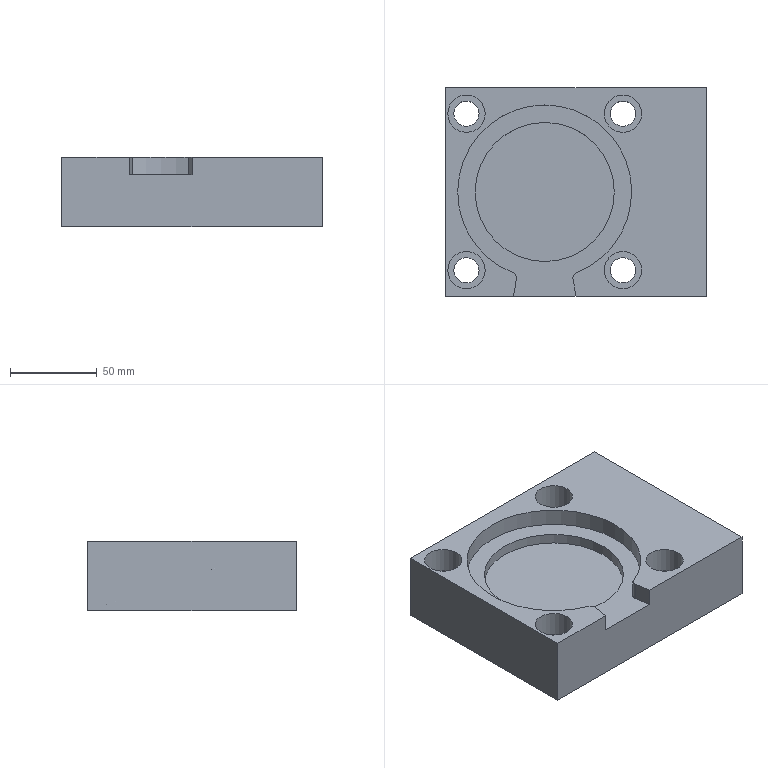NC program | NX | posted with a generic post | part box 150 x 120 x 40 mm
Lines 32 to 853 of 1997:
(HOLE_MILLING , TOOL : D10)
N56 T10 M6
N58 G54
N60 G17 G0 G90 X-63. Y45. S9500 M3
N62 G43 Z30. H10
N64 Z0.5
N66 G94 G3 X-61.563 Y43.563 R1.438 F1500.
N68 X-60.125 Y45. R1.438
N70 X-60.125 Y45. Z-0.5 I-2.875 J0.
N72 X-60.125 Y45. Z-1.5 I-2.875 J0.
N74 X-60.125 Y45. Z-2.5 I-2.875 J0.
N76 X-60.125 Y45. Z-3.5 I-2.875 J0.
N78 X-60.125 Y45. Z-4.5 I-2.875 J0.
N80 X-60.125 Y45. Z-5.5 I-2.875 J0.
N82 X-60.125 Y45. Z-6.5 I-2.875 J0.
N84 X-60.125 Y45. Z-7.5 I-2.875 J0.
N86 X-60.125 Y45. Z-8.5 I-2.875 J0.
N88 X-60.125 Y45. Z-9.5 I-2.875 J0.
N90 X-60.125 Y45. Z-10.5 I-2.875 J0.
N92 X-60.125 Y45. Z-11.5 I-2.875 J0.
N94 X-60.125 Y45. Z-12.5 I-2.875 J0.
N96 X-60.125 Y45. Z-13.5 I-2.875 J0.
N98 X-60.125 Y45. Z-14.5 I-2.875 J0.
N100 X-65.875 Y45. Z-15. I-2.875 J0.
N102 X-63. Y42.125 R2.875
N104 X-65.875 Y45. R-2.875
N106 X-64.438 Y43.563 R1.438
N108 X-63. Y45. R1.438
N110 G0 Z0.5
N112 G3 X-60.125 Y42.125 R2.875
N114 X-57.25 Y45. R2.875
N116 X-57.25 Y45. Z-0.5 I-5.75 J0.
N118 X-57.25 Y45. Z-1.5 I-5.75 J0.
N120 X-57.25 Y45. Z-2.5 I-5.75 J0.
N122 X-57.25 Y45. Z-3.5 I-5.75 J0.
N124 X-57.25 Y45. Z-4.5 I-5.75 J0.
N126 X-57.25 Y45. Z-5.5 I-5.75 J0.
N128 X-57.25 Y45. Z-6.5 I-5.75 J0.
N130 X-57.25 Y45. Z-7.5 I-5.75 J0.
N132 X-57.25 Y45. Z-8.5 I-5.75 J0.
N134 X-57.25 Y45. Z-9.5 I-5.75 J0.
N136 X-57.25 Y45. Z-10.5 I-5.75 J0.
N138 X-57.25 Y45. Z-11.5 I-5.75 J0.
N140 X-57.25 Y45. Z-12.5 I-5.75 J0.
N142 X-57.25 Y45. Z-13.5 I-5.75 J0.
N144 X-57.25 Y45. Z-14.5 I-5.75 J0.
N146 X-68.75 Y45. Z-15. I-5.75 J0.
N148 X-63. Y39.25 R5.75
N150 X-68.75 Y45. R-5.75
N152 X-65.875 Y42.125 R2.875
N154 X-63. Y45. R2.875
N156 G0 Z30.
N158 X27.
N160 Z0.5
N162 G3 X28.438 Y43.563 R1.438
N164 X29.875 Y45. R1.438
N166 X29.875 Y45. Z-0.5 I-2.875 J0.
N168 X29.875 Y45. Z-1.5 I-2.875 J0.
N170 X29.875 Y45. Z-2.5 I-2.875 J0.
N172 X29.875 Y45. Z-3.5 I-2.875 J0.
N174 X29.875 Y45. Z-4.5 I-2.875 J0.
N176 X29.875 Y45. Z-5.5 I-2.875 J0.
N178 X29.875 Y45. Z-6.5 I-2.875 J0.
N180 X29.875 Y45. Z-7.5 I-2.875 J0.
N182 X29.875 Y45. Z-8.5 I-2.875 J0.
N184 X29.875 Y45. Z-9.5 I-2.875 J0.
N186 X29.875 Y45. Z-10.5 I-2.875 J0.
N188 X29.875 Y45. Z-11.5 I-2.875 J0.
N190 X29.875 Y45. Z-12.5 I-2.875 J0.
N192 X29.875 Y45. Z-13.5 I-2.875 J0.
N194 X29.875 Y45. Z-14.5 I-2.875 J0.
N196 X24.125 Y45. Z-15. I-2.875 J0.
N198 X27. Y42.125 R2.875
N200 X24.125 Y45. R-2.875
N202 X25.563 Y43.563 R1.438
N204 X27. Y45. R1.438
N206 G0 Z0.5
N208 G3 X29.875 Y42.125 R2.875
N210 X32.75 Y45. R2.875
N212 X32.75 Y45. Z-0.5 I-5.75 J0.
N214 X32.75 Y45. Z-1.5 I-5.75 J0.
N216 X32.75 Y45. Z-2.5 I-5.75 J0.
N218 X32.75 Y45. Z-3.5 I-5.75 J0.
N220 X32.75 Y45. Z-4.5 I-5.75 J0.
N222 X32.75 Y45. Z-5.5 I-5.75 J0.
N224 X32.75 Y45. Z-6.5 I-5.75 J0.
N226 X32.75 Y45. Z-7.5 I-5.75 J0.
N228 X32.75 Y45. Z-8.5 I-5.75 J0.
N230 X32.75 Y45. Z-9.5 I-5.75 J0.
N232 X32.75 Y45. Z-10.5 I-5.75 J0.
N234 X32.75 Y45. Z-11.5 I-5.75 J0.
N236 X32.75 Y45. Z-12.5 I-5.75 J0.
N238 X32.75 Y45. Z-13.5 I-5.75 J0.
N240 X32.75 Y45. Z-14.5 I-5.75 J0.
N242 X21.25 Y45. Z-15. I-5.75 J0.
N244 X27. Y39.25 R5.75
N246 X21.25 Y45. R-5.75
N248 X24.125 Y42.125 R2.875
N250 X27. Y45. R2.875
N252 G0 Z30.
N254 Y-45.
N256 Z0.5
N258 G3 X28.438 Y-46.438 R1.438
N260 X29.875 Y-45. R1.438
N262 X29.875 Y-45. Z-0.5 I-2.875 J0.
N264 X29.875 Y-45. Z-1.5 I-2.875 J0.
N266 X29.875 Y-45. Z-2.5 I-2.875 J0.
N268 X29.875 Y-45. Z-3.5 I-2.875 J0.
N270 X29.875 Y-45. Z-4.5 I-2.875 J0.
N272 X29.875 Y-45. Z-5.5 I-2.875 J0.
N274 X29.875 Y-45. Z-6.5 I-2.875 J0.
N276 X29.875 Y-45. Z-7.5 I-2.875 J0.
N278 X29.875 Y-45. Z-8.5 I-2.875 J0.
N280 X29.875 Y-45. Z-9.5 I-2.875 J0.
N282 X29.875 Y-45. Z-10.5 I-2.875 J0.
N284 X29.875 Y-45. Z-11.5 I-2.875 J0.
N286 X29.875 Y-45. Z-12.5 I-2.875 J0.
N288 X29.875 Y-45. Z-13.5 I-2.875 J0.
N290 X29.875 Y-45. Z-14.5 I-2.875 J0.
N292 X24.125 Y-45. Z-15. I-2.875 J0.
N294 X27. Y-47.875 R2.875
N296 X24.125 Y-45. R-2.875
N298 X25.563 Y-46.438 R1.438
N300 X27. Y-45. R1.438
N302 G0 Z0.5
N304 G3 X29.875 Y-47.875 R2.875
N306 X32.75 Y-45. R2.875
N308 X32.75 Y-45. Z-0.5 I-5.75 J0.
N310 X32.75 Y-45. Z-1.5 I-5.75 J0.
N312 X32.75 Y-45. Z-2.5 I-5.75 J0.
N314 X32.75 Y-45. Z-3.5 I-5.75 J0.
N316 X32.75 Y-45. Z-4.5 I-5.75 J0.
N318 X32.75 Y-45. Z-5.5 I-5.75 J0.
N320 X32.75 Y-45. Z-6.5 I-5.75 J0.
N322 X32.75 Y-45. Z-7.5 I-5.75 J0.
N324 X32.75 Y-45. Z-8.5 I-5.75 J0.
N326 X32.75 Y-45. Z-9.5 I-5.75 J0.
N328 X32.75 Y-45. Z-10.5 I-5.75 J0.
N330 X32.75 Y-45. Z-11.5 I-5.75 J0.
N332 X32.75 Y-45. Z-12.5 I-5.75 J0.
N334 X32.75 Y-45. Z-13.5 I-5.75 J0.
N336 X32.75 Y-45. Z-14.5 I-5.75 J0.
N338 X21.25 Y-45. Z-15. I-5.75 J0.
N340 X27. Y-50.75 R5.75
N342 X21.25 Y-45. R-5.75
N344 X24.125 Y-47.875 R2.875
N346 X27. Y-45. R2.875
N348 G0 Z30.
N350 X-63.
N352 Z0.5
N354 G3 X-61.563 Y-46.438 R1.438
N356 X-60.125 Y-45. R1.438
N358 X-60.125 Y-45. Z-0.5 I-2.875 J0.
N360 X-60.125 Y-45. Z-1.5 I-2.875 J0.
N362 X-60.125 Y-45. Z-2.5 I-2.875 J0.
N364 X-60.125 Y-45. Z-3.5 I-2.875 J0.
N366 X-60.125 Y-45. Z-4.5 I-2.875 J0.
N368 X-60.125 Y-45. Z-5.5 I-2.875 J0.
N370 X-60.125 Y-45. Z-6.5 I-2.875 J0.
N372 X-60.125 Y-45. Z-7.5 I-2.875 J0.
N374 X-60.125 Y-45. Z-8.5 I-2.875 J0.
N376 X-60.125 Y-45. Z-9.5 I-2.875 J0.
N378 X-60.125 Y-45. Z-10.5 I-2.875 J0.
N380 X-60.125 Y-45. Z-11.5 I-2.875 J0.
N382 X-60.125 Y-45. Z-12.5 I-2.875 J0.
N384 X-60.125 Y-45. Z-13.5 I-2.875 J0.
N386 X-60.125 Y-45. Z-14.5 I-2.875 J0.
N388 X-65.875 Y-45. Z-15. I-2.875 J0.
N390 X-63. Y-47.875 R2.875
N392 X-65.875 Y-45. R-2.875
N394 X-64.438 Y-46.438 R1.438
N396 X-63. Y-45. R1.438
N398 G0 Z0.5
N400 G3 X-60.125 Y-47.875 R2.875
N402 X-57.25 Y-45. R2.875
N404 X-57.25 Y-45. Z-0.5 I-5.75 J0.
N406 X-57.25 Y-45. Z-1.5 I-5.75 J0.
N408 X-57.25 Y-45. Z-2.5 I-5.75 J0.
N410 X-57.25 Y-45. Z-3.5 I-5.75 J0.
N412 X-57.25 Y-45. Z-4.5 I-5.75 J0.
N414 X-57.25 Y-45. Z-5.5 I-5.75 J0.
N416 X-57.25 Y-45. Z-6.5 I-5.75 J0.
N418 X-57.25 Y-45. Z-7.5 I-5.75 J0.
N420 X-57.25 Y-45. Z-8.5 I-5.75 J0.
N422 X-57.25 Y-45. Z-9.5 I-5.75 J0.
N424 X-57.25 Y-45. Z-10.5 I-5.75 J0.
N426 X-57.25 Y-45. Z-11.5 I-5.75 J0.
N428 X-57.25 Y-45. Z-12.5 I-5.75 J0.
N430 X-57.25 Y-45. Z-13.5 I-5.75 J0.
N432 X-57.25 Y-45. Z-14.5 I-5.75 J0.
N434 X-68.75 Y-45. Z-15. I-5.75 J0.
N436 X-63. Y-50.75 R5.75
N438 X-68.75 Y-45. R-5.75
N440 X-65.875 Y-47.875 R2.875
N442 X-63. Y-45. R2.875
N444 G0 Z30.
(FLOOR_WALL , TOOL : D10)
N446 X-16.17 Y2.26
N448 Z1.5
N450 G1 X-16.818 Y2.681 Z1.459 F1000.
N452 X-17.725 Y2.917 Z1.41
N454 X-18.66 Y2.855 Z1.361
N456 X-19.049 Y2.703 Z1.339
N458 X-19.439 Y2.552 Z1.317
N460 X-20.171 Y1.967 Z1.268
N462 X-20.681 Y1.182 Z1.219
N464 X-20.917 Y0.275 Z1.17
N466 X-20.855 Y-0.66 Z1.121
N468 X-20.703 Y-1.049 Z1.099
N470 X-20.552 Y-1.439 Z1.077
N472 X-20.072 Y-2.072 Z1.036
N474 X-19.439 Y-2.552 Z0.994
N476 X-18. Y-3.125 Z0.913
N478 X-16.561 Y-2.552 Z0.832
N480 X-15.829 Y-1.967 Z0.783
N482 X-15.319 Y-1.182 Z0.733
N484 X-15.083 Y-0.275 Z0.684
N486 X-15.145 Y0.66 Z0.635
N488 X-15.297 Y1.049 Z0.613
N490 X-15.448 Y1.439 Z0.591
N492 X-16.033 Y2.171 Z0.542
N494 X-16.818 Y2.681 Z0.493
N496 X-17.725 Y2.917 Z0.444
N498 X-18.66 Y2.855 Z0.395
N500 X-19.049 Y2.703 Z0.373
N502 X-19.439 Y2.552 Z0.351
N504 X-20.171 Y1.967 Z0.302
N506 X-20.681 Y1.182 Z0.253
N508 X-20.917 Y0.275 Z0.204
N510 X-20.855 Y-0.66 Z0.155
N512 X-20.703 Y-1.049 Z0.133
N514 X-20.552 Y-1.439 Z0.111
N516 X-20.072 Y-2.072 Z0.069
N518 X-19.439 Y-2.552 Z0.028
N520 X-18. Y-3.125 Z-0.053
N522 X-16.561 Y-2.552 Z-0.135
N524 X-15.829 Y-1.967 Z-0.184
N526 X-15.319 Y-1.182 Z-0.233
N528 X-15.083 Y-0.275 Z-0.282
N530 X-15.145 Y0.66 Z-0.331
N532 X-15.297 Y1.049 Z-0.353
N534 X-15.448 Y1.439 Z-0.375
N536 X-16.033 Y2.171 Z-0.424
N538 X-16.818 Y2.681 Z-0.473
N540 X-17.725 Y2.917 Z-0.522
N542 X-18.66 Y2.855 Z-0.571
N544 X-19.049 Y2.703 Z-0.593
N546 X-19.439 Y2.552 Z-0.615
N548 X-20.171 Y1.967 Z-0.664
N550 X-20.681 Y1.182 Z-0.713
N552 X-20.917 Y0.275 Z-0.762
N554 X-20.855 Y-0.66 Z-0.811
N556 X-20.703 Y-1.049 Z-0.833
N558 X-20.552 Y-1.439 Z-0.855
N560 X-20.072 Y-2.072 Z-0.897
N562 X-19.439 Y-2.552 Z-0.938
N564 X-18.524 Y-2.911 Z-0.99
N566 G2 X-18. Y-3.125 R50.1 F3500.
N568 X-16.951 Y-2.703 R50.1
N570 G3 X-19.049 Y-2.703 R-2.9
N572 G2 X-18.524 Y-2.911 R50.1
N574 G1 X-20.758 Y-8.48
N576 G2 X-18. Y-9.697 R44.1
N578 X-14.779 Y-8.297 R44.1
N580 G3 X-21.221 Y-8.297 R-8.9
N582 G2 X-20.758 Y-8.48 R44.1
N584 G1 X-22.992 Y-14.048
N586 G2 X-18. Y-16.487 R38.1
N588 X-12.608 Y-13.89 R38.1
N590 G3 X-23.392 Y-13.89 R-14.9
N592 G2 X-22.992 Y-14.048 R38.1
N594 G1 X-25.226 Y-19.617
N596 G2 X-18. Y-23.667 R32.1
N598 X-10.437 Y-19.484 R32.1
N600 G3 X-25.563 Y-19.484 R-20.9
N602 G2 X-25.226 Y-19.617 R32.1
N604 G1 X-27.46 Y-25.185
N606 G2 X-18. Y-31.706 R26.1
N608 X-8.266 Y-25.077 R26.1
N610 G3 X-27.734 Y-25.077 R-26.9
N612 G2 X-27.46 Y-25.185 R26.1
N614 G1 X-29.694 Y-30.754
N616 G2 X-18. Y-43.393 R20.1
N618 G1 Y-52.243
N620 Y-43.393
N622 G2 X-6.095 Y-30.67 R20.1
N624 G3 X-29.905 Y-30.67 R-32.9
N626 G2 X-29.694 Y-30.754 R20.1
N628 G1 X-31.928 Y-36.322
N630 G2 X-23.293 Y-51.857 R14.1
N632 G1 X-24.552 Y-59.
N634 X-11.448
N636 X-12.707 Y-51.856
N638 G2 X-3.924 Y-36.264 R14.1
N640 G3 X-32.076 Y-36.264 R-38.9
N642 G1 X-31.928 Y-36.322
N644 X-34.163 Y-41.891
N646 G2 X-29.202 Y-50.815 R8.1
N648 G1 X-31.703 Y-65.
N650 X-4.297
N652 X-6.798 Y-50.815
N654 G2 X-1.752 Y-41.857 R8.1
N656 G3 X-34.248 Y-41.857 R-44.9
N658 G1 X-34.163 Y-41.891
N660 Z0.51
N662 G0 Z3.
N664 X-16.17 Y2.26
N666 Z0.51
N668 G1 X-16.818 Y2.681 Z0.469 F1000.
N670 X-17.725 Y2.917 Z0.42
N672 X-18.66 Y2.855 Z0.371
N674 X-19.049 Y2.703 Z0.349
N676 X-19.439 Y2.552 Z0.327
N678 X-20.171 Y1.967 Z0.278
N680 X-20.681 Y1.182 Z0.229
N682 X-20.917 Y0.275 Z0.18
N684 X-20.855 Y-0.66 Z0.131
N686 X-20.703 Y-1.049 Z0.109
N688 X-20.552 Y-1.439 Z0.087
N690 X-20.072 Y-2.072 Z0.046
N692 X-19.439 Y-2.552 Z0.004
N694 X-18. Y-3.125 Z-0.077
N696 X-16.561 Y-2.552 Z-0.158
N698 X-15.829 Y-1.967 Z-0.207
N700 X-15.319 Y-1.182 Z-0.257
N702 X-15.083 Y-0.275 Z-0.306
N704 X-15.145 Y0.66 Z-0.355
N706 X-15.297 Y1.049 Z-0.377
N708 X-15.448 Y1.439 Z-0.399
N710 X-16.033 Y2.171 Z-0.448
N712 X-16.818 Y2.681 Z-0.497
N714 X-17.725 Y2.917 Z-0.546
N716 X-18.66 Y2.855 Z-0.595
N718 X-19.049 Y2.703 Z-0.617
N720 X-19.439 Y2.552 Z-0.639
N722 X-20.171 Y1.967 Z-0.688
N724 X-20.681 Y1.182 Z-0.737
N726 X-20.917 Y0.275 Z-0.786
N728 X-20.855 Y-0.66 Z-0.835
N730 X-20.703 Y-1.049 Z-0.857
N732 X-20.552 Y-1.439 Z-0.879
N734 X-20.072 Y-2.072 Z-0.921
N736 X-19.439 Y-2.552 Z-0.962
N738 X-18. Y-3.125 Z-1.043
N740 X-16.561 Y-2.552 Z-1.125
N742 X-15.829 Y-1.967 Z-1.174
N744 X-15.319 Y-1.182 Z-1.223
N746 X-15.083 Y-0.275 Z-1.272
N748 X-15.145 Y0.66 Z-1.321
N750 X-15.297 Y1.049 Z-1.343
N752 X-15.448 Y1.439 Z-1.365
N754 X-16.033 Y2.171 Z-1.414
N756 X-16.818 Y2.681 Z-1.463
N758 X-17.725 Y2.917 Z-1.512
N760 X-18.66 Y2.855 Z-1.561
N762 X-19.049 Y2.703 Z-1.583
N764 X-19.439 Y2.552 Z-1.605
N766 X-20.171 Y1.967 Z-1.654
N768 X-20.681 Y1.182 Z-1.703
N770 X-20.917 Y0.275 Z-1.752
N772 X-20.855 Y-0.66 Z-1.801
N774 X-20.703 Y-1.049 Z-1.823
N776 X-20.552 Y-1.439 Z-1.845
N778 X-20.072 Y-2.072 Z-1.887
N780 X-19.439 Y-2.552 Z-1.928
N782 X-18.524 Y-2.911 Z-1.98
N784 G2 X-18. Y-3.125 R50.1 F3500.
N786 X-16.951 Y-2.703 R50.1
N788 G3 X-19.049 Y-2.703 R-2.9
N790 G2 X-18.524 Y-2.911 R50.1
N792 G1 X-20.758 Y-8.48
N794 G2 X-18. Y-9.697 R44.1
N796 X-14.779 Y-8.297 R44.1
N798 G3 X-21.221 Y-8.297 R-8.9
N800 G2 X-20.758 Y-8.48 R44.1
N802 G1 X-22.992 Y-14.048
N804 G2 X-18. Y-16.487 R38.1
N806 X-12.608 Y-13.89 R38.1
N808 G3 X-23.392 Y-13.89 R-14.9
N810 G2 X-22.992 Y-14.048 R38.1
N812 G1 X-25.226 Y-19.617
N814 G2 X-18. Y-23.667 R32.1
N816 X-10.437 Y-19.484 R32.1
N818 G3 X-25.563 Y-19.484 R-20.9
N820 G2 X-25.226 Y-19.617 R32.1
N822 G1 X-27.46 Y-25.185
N824 G2 X-18. Y-31.706 R26.1
N826 X-8.266 Y-25.077 R26.1
N828 G3 X-27.734 Y-25.077 R-26.9
N830 G2 X-27.46 Y-25.185 R26.1
N832 G1 X-29.694 Y-30.754
N834 G2 X-18. Y-43.393 R20.1
N836 G1 Y-52.243
N838 Y-43.393
N840 G2 X-6.095 Y-30.67 R20.1
N842 G3 X-29.905 Y-30.67 R-32.9
N844 G2 X-29.694 Y-30.754 R20.1
N846 G1 X-31.928 Y-36.322
N848 G2 X-23.293 Y-51.857 R14.1
N850 G1 X-24.552 Y-59.
N852 X-11.448
N854 X-12.707 Y-51.856
N856 G2 X-3.924 Y-36.264 R14.1
N858 G3 X-32.076 Y-36.264 R-38.9
N860 G1 X-31.928 Y-36.322
N862 X-34.163 Y-41.891
N864 G2 X-29.202 Y-50.815 R8.1
N866 G1 X-31.703 Y-65.
N868 X-4.297
N870 X-6.798 Y-50.815
N872 G2 X-1.752 Y-41.857 R8.1
N874 G3 X-34.248 Y-41.857 R-44.9
N876 G1 X-34.163 Y-41.891
N878 Z-0.48
N880 G0 Z2.01
N882 X-16.17 Y2.26
N884 Z-0.48
N886 G1 X-16.818 Y2.681 Z-0.521 F1000.
N888 X-17.725 Y2.917 Z-0.57
N890 X-18.66 Y2.855 Z-0.619
N892 X-19.049 Y2.703 Z-0.641
N894 X-19.439 Y2.552 Z-0.663
N896 X-20.171 Y1.967 Z-0.712
N898 X-20.681 Y1.182 Z-0.761
N900 X-20.917 Y0.275 Z-0.81
N902 X-20.855 Y-0.66 Z-0.859
N904 X-20.703 Y-1.049 Z-0.881
N906 X-20.552 Y-1.439 Z-0.903
N908 X-20.072 Y-2.072 Z-0.944
N910 X-19.439 Y-2.552 Z-0.986
N912 X-18. Y-3.125 Z-1.067
N914 X-16.561 Y-2.552 Z-1.148
N916 X-15.829 Y-1.967 Z-1.197
N918 X-15.319 Y-1.182 Z-1.247
N920 X-15.083 Y-0.275 Z-1.296
N922 X-15.145 Y0.66 Z-1.345
N924 X-15.297 Y1.049 Z-1.367
N926 X-15.448 Y1.439 Z-1.389
N928 X-16.033 Y2.171 Z-1.438
N930 X-16.818 Y2.681 Z-1.487
N932 X-17.725 Y2.917 Z-1.536
N934 X-18.66 Y2.855 Z-1.585
N936 X-19.049 Y2.703 Z-1.607
N938 X-19.439 Y2.552 Z-1.629
N940 X-20.171 Y1.967 Z-1.678
N942 X-20.681 Y1.182 Z-1.727
N944 X-20.917 Y0.275 Z-1.776
N946 X-20.855 Y-0.66 Z-1.825
N948 X-20.703 Y-1.049 Z-1.847
N950 X-20.552 Y-1.439 Z-1.869
N952 X-20.072 Y-2.072 Z-1.911
N954 X-19.439 Y-2.552 Z-1.952
N956 X-18. Y-3.125 Z-2.033
N958 X-16.561 Y-2.552 Z-2.115
N960 X-15.829 Y-1.967 Z-2.164
N962 X-15.319 Y-1.182 Z-2.213
N964 X-15.083 Y-0.275 Z-2.262
N966 X-15.145 Y0.66 Z-2.311
N968 X-15.297 Y1.049 Z-2.333
N970 X-15.448 Y1.439 Z-2.355
N972 X-16.033 Y2.171 Z-2.404
N974 X-16.818 Y2.681 Z-2.453
N976 X-17.725 Y2.917 Z-2.502
N978 X-18.66 Y2.855 Z-2.551
N980 X-19.049 Y2.703 Z-2.573
N982 X-19.439 Y2.552 Z-2.595
N984 X-20.171 Y1.967 Z-2.644
N986 X-20.681 Y1.182 Z-2.693
N988 X-20.917 Y0.275 Z-2.742
N990 X-20.855 Y-0.66 Z-2.791
N992 X-20.703 Y-1.049 Z-2.813
N994 X-20.552 Y-1.439 Z-2.835
N996 X-20.072 Y-2.072 Z-2.877
N998 X-19.439 Y-2.552 Z-2.918
N1000 X-18.524 Y-2.911 Z-2.97
N1002 G2 X-18. Y-3.125 R50.1 F3500.
N1004 X-16.951 Y-2.703 R50.1
N1006 G3 X-19.049 Y-2.703 R-2.9
N1008 G2 X-18.524 Y-2.911 R50.1
N1010 G1 X-20.758 Y-8.48
N1012 G2 X-18. Y-9.697 R44.1
N1014 X-14.779 Y-8.297 R44.1
N1016 G3 X-21.221 Y-8.297 R-8.9
N1018 G2 X-20.758 Y-8.48 R44.1
N1020 G1 X-22.992 Y-14.048
N1022 G2 X-18. Y-16.487 R38.1
N1024 X-12.608 Y-13.89 R38.1
N1026 G3 X-23.392 Y-13.89 R-14.9
N1028 G2 X-22.992 Y-14.048 R38.1
N1030 G1 X-25.226 Y-19.617
N1032 G2 X-18. Y-23.667 R32.1
N1034 X-10.437 Y-19.484 R32.1
N1036 G3 X-25.563 Y-19.484 R-20.9
N1038 G2 X-25.226 Y-19.617 R32.1
N1040 G1 X-27.46 Y-25.185
N1042 G2 X-18. Y-31.706 R26.1
N1044 X-8.266 Y-25.077 R26.1
N1046 G3 X-27.734 Y-25.077 R-26.9
N1048 G2 X-27.46 Y-25.185 R26.1
N1050 G1 X-29.694 Y-30.754
N1052 G2 X-18. Y-43.393 R20.1
N1054 G1 Y-52.243
N1056 Y-43.393
N1058 G2 X-6.095 Y-30.67 R20.1
N1060 G3 X-29.905 Y-30.67 R-32.9
N1062 G2 X-29.694 Y-30.754 R20.1
N1064 G1 X-31.928 Y-36.322
N1066 G2 X-23.293 Y-51.857 R14.1
N1068 G1 X-24.552 Y-59.
N1070 X-11.448
N1072 X-12.707 Y-51.856
N1074 G2 X-3.924 Y-36.264 R14.1
N1076 G3 X-32.076 Y-36.264 R-38.9
N1078 G1 X-31.928 Y-36.322
N1080 X-34.163 Y-41.891
N1082 G2 X-29.202 Y-50.815 R8.1
N1084 G1 X-31.703 Y-65.
N1086 X-4.297
N1088 X-6.798 Y-50.815
N1090 G2 X-1.752 Y-41.857 R8.1
N1092 G3 X-34.248 Y-41.857 R-44.9
N1094 G1 X-34.163 Y-41.891
N1096 Z-1.47
N1098 G0 Z1.02
N1100 X-16.17 Y2.26
N1102 Z-1.47
N1104 G1 X-16.818 Y2.681 Z-1.511 F1000.
N1106 X-17.725 Y2.917 Z-1.56
N1108 X-18.66 Y2.855 Z-1.609
N1110 X-19.049 Y2.703 Z-1.631
N1112 X-19.439 Y2.552 Z-1.653
N1114 X-20.171 Y1.967 Z-1.702
N1116 X-20.681 Y1.182 Z-1.751
N1118 X-20.917 Y0.275 Z-1.8
N1120 X-20.855 Y-0.66 Z-1.849
N1122 X-20.703 Y-1.049 Z-1.871
N1124 X-20.552 Y-1.439 Z-1.893
N1126 X-20.072 Y-2.072 Z-1.934
N1128 X-19.439 Y-2.552 Z-1.976
N1130 X-18. Y-3.125 Z-2.057
N1132 X-16.561 Y-2.552 Z-2.138
N1134 X-15.829 Y-1.967 Z-2.187
N1136 X-15.319 Y-1.182 Z-2.237
N1138 X-15.083 Y-0.275 Z-2.286
N1140 X-15.145 Y0.66 Z-2.335
N1142 X-15.297 Y1.049 Z-2.357
N1144 X-15.448 Y1.439 Z-2.379
N1146 X-16.033 Y2.171 Z-2.428
N1148 X-16.818 Y2.681 Z-2.477
N1150 X-17.725 Y2.917 Z-2.526
N1152 X-18.66 Y2.855 Z-2.575
N1154 X-19.049 Y2.703 Z-2.597
N1156 X-19.439 Y2.552 Z-2.619
N1158 X-20.171 Y1.967 Z-2.668
N1160 X-20.681 Y1.182 Z-2.717
N1162 X-20.917 Y0.275 Z-2.766
N1164 X-20.855 Y-0.66 Z-2.815
N1166 X-20.703 Y-1.049 Z-2.837
N1168 X-20.552 Y-1.439 Z-2.859
N1170 X-20.072 Y-2.072 Z-2.901
N1172 X-19.439 Y-2.552 Z-2.942
N1174 X-18. Y-3.125 Z-3.023
N1176 X-16.561 Y-2.552 Z-3.105
N1178 X-15.829 Y-1.967 Z-3.154
N1180 X-15.319 Y-1.182 Z-3.203
N1182 X-15.083 Y-0.275 Z-3.252
N1184 X-15.145 Y0.66 Z-3.301
N1186 X-15.297 Y1.049 Z-3.323
N1188 X-15.448 Y1.439 Z-3.345
N1190 X-16.033 Y2.171 Z-3.394
N1192 X-16.818 Y2.681 Z-3.443
N1194 X-17.725 Y2.917 Z-3.492
N1196 X-18.66 Y2.855 Z-3.541
N1198 X-19.049 Y2.703 Z-3.563
N1200 X-19.439 Y2.552 Z-3.585
N1202 X-20.171 Y1.967 Z-3.634
N1204 X-20.681 Y1.182 Z-3.683
N1206 X-20.917 Y0.275 Z-3.732
N1208 X-20.855 Y-0.66 Z-3.781
N1210 X-20.703 Y-1.049 Z-3.803
N1212 X-20.552 Y-1.439 Z-3.825
N1214 X-20.072 Y-2.072 Z-3.867
N1216 X-19.439 Y-2.552 Z-3.908
N1218 X-18.524 Y-2.911 Z-3.96
N1220 G2 X-18. Y-3.125 R50.1 F3500.
N1222 X-16.951 Y-2.703 R50.1
N1224 G3 X-19.049 Y-2.703 R-2.9
N1226 G2 X-18.524 Y-2.911 R50.1
N1228 G1 X-20.758 Y-8.48
N1230 G2 X-18. Y-9.697 R44.1
N1232 X-14.779 Y-8.297 R44.1
N1234 G3 X-21.221 Y-8.297 R-8.9
N1236 G2 X-20.758 Y-8.48 R44.1
N1238 G1 X-22.992 Y-14.048
N1240 G2 X-18. Y-16.487 R38.1
N1242 X-12.608 Y-13.89 R38.1
N1244 G3 X-23.392 Y-13.89 R-14.9
N1246 G2 X-22.992 Y-14.048 R38.1
N1248 G1 X-25.226 Y-19.617
N1250 G2 X-18. Y-23.667 R32.1
N1252 X-10.437 Y-19.484 R32.1
N1254 G3 X-25.563 Y-19.484 R-20.9
N1256 G2 X-25.226 Y-19.617 R32.1
N1258 G1 X-27.46 Y-25.185
N1260 G2 X-18. Y-31.706 R26.1
N1262 X-8.266 Y-25.077 R26.1
N1264 G3 X-27.734 Y-25.077 R-26.9
N1266 G2 X-27.46 Y-25.185 R26.1
N1268 G1 X-29.694 Y-30.754
N1270 G2 X-18. Y-43.393 R20.1
N1272 G1 Y-52.243
N1274 Y-43.393
N1276 G2 X-6.095 Y-30.67 R20.1
N1278 G3 X-29.905 Y-30.67 R-32.9
N1280 G2 X-29.694 Y-30.754 R20.1
N1282 G1 X-31.928 Y-36.322
N1284 G2 X-23.293 Y-51.857 R14.1
N1286 G1 X-24.552 Y-59.
N1288 X-11.448
N1290 X-12.707 Y-51.856
N1292 G2 X-3.924 Y-36.264 R14.1
N1294 G3 X-32.076 Y-36.264 R-38.9
N1296 G1 X-31.928 Y-36.322
N1298 X-34.163 Y-41.891
N1300 G2 X-29.202 Y-50.815 R8.1
N1302 G1 X-31.703 Y-65.
N1304 X-4.297
N1306 X-6.798 Y-50.815
N1308 G2 X-1.752 Y-41.857 R8.1
N1310 G3 X-34.248 Y-41.857 R-44.9
N1312 G1 X-34.163 Y-41.891
N1314 Z-2.46
N1316 G0 Z0.03
N1318 X-16.17 Y2.26
N1320 Z-2.46
N1322 G1 X-16.818 Y2.681 Z-2.501 F1000.
N1324 X-17.725 Y2.917 Z-2.55
N1326 X-18.66 Y2.855 Z-2.599
N1328 X-19.049 Y2.703 Z-2.621
N1330 X-19.439 Y2.552 Z-2.643
N1332 X-20.171 Y1.967 Z-2.692
N1334 X-20.681 Y1.182 Z-2.741
N1336 X-20.917 Y0.275 Z-2.79
N1338 X-20.855 Y-0.66 Z-2.839
N1340 X-20.703 Y-1.049 Z-2.861
N1342 X-20.552 Y-1.439 Z-2.883
N1344 X-20.072 Y-2.072 Z-2.924
N1346 X-19.439 Y-2.552 Z-2.966
N1348 X-18. Y-3.125 Z-3.047
N1350 X-16.561 Y-2.552 Z-3.128
N1352 X-15.829 Y-1.967 Z-3.177
N1354 X-15.319 Y-1.182 Z-3.227
N1356 X-15.083 Y-0.275 Z-3.276
N1358 X-15.145 Y0.66 Z-3.325
N1360 X-15.297 Y1.049 Z-3.347
N1362 X-15.448 Y1.439 Z-3.369
N1364 X-16.033 Y2.171 Z-3.418
N1366 X-16.818 Y2.681 Z-3.467
N1368 X-17.725 Y2.917 Z-3.516
N1370 X-18.66 Y2.855 Z-3.565
N1372 X-19.049 Y2.703 Z-3.587
N1374 X-19.439 Y2.552 Z-3.609
N1376 X-20.171 Y1.967 Z-3.658
N1378 X-20.681 Y1.182 Z-3.707
N1380 X-20.917 Y0.275 Z-3.756
N1382 X-20.855 Y-0.66 Z-3.805
N1384 X-20.703 Y-1.049 Z-3.827
N1386 X-20.552 Y-1.439 Z-3.849
N1388 X-20.072 Y-2.072 Z-3.891
N1390 X-19.439 Y-2.552 Z-3.932
N1392 X-18. Y-3.125 Z-4.013
N1394 X-16.561 Y-2.552 Z-4.095
N1396 X-15.829 Y-1.967 Z-4.144
N1398 X-15.319 Y-1.182 Z-4.193
N1400 X-15.083 Y-0.275 Z-4.242
N1402 X-15.145 Y0.66 Z-4.291
N1404 X-15.297 Y1.049 Z-4.313
N1406 X-15.448 Y1.439 Z-4.335
N1408 X-16.033 Y2.171 Z-4.384
N1410 X-16.818 Y2.681 Z-4.433
N1412 X-17.725 Y2.917 Z-4.482
N1414 X-18.66 Y2.855 Z-4.531
N1416 X-19.049 Y2.703 Z-4.553
N1418 X-19.439 Y2.552 Z-4.575
N1420 X-20.171 Y1.967 Z-4.624
N1422 X-20.681 Y1.182 Z-4.673
N1424 X-20.917 Y0.275 Z-4.722
N1426 X-20.855 Y-0.66 Z-4.771
N1428 X-20.703 Y-1.049 Z-4.793
N1430 X-20.552 Y-1.439 Z-4.815
N1432 X-20.072 Y-2.072 Z-4.857
N1434 X-19.439 Y-2.552 Z-4.898
N1436 X-18.524 Y-2.911 Z-4.95
N1438 G2 X-18. Y-3.125 R50.1 F3500.
N1440 X-16.951 Y-2.703 R50.1
N1442 G3 X-19.049 Y-2.703 R-2.9
N1444 G2 X-18.524 Y-2.911 R50.1
N1446 G1 X-20.758 Y-8.48
N1448 G2 X-18. Y-9.697 R44.1
N1450 X-14.779 Y-8.297 R44.1
N1452 G3 X-21.221 Y-8.297 R-8.9
N1454 G2 X-20.758 Y-8.48 R44.1
N1456 G1 X-22.992 Y-14.048
N1458 G2 X-18. Y-16.487 R38.1
N1460 X-12.608 Y-13.89 R38.1
N1462 G3 X-23.392 Y-13.89 R-14.9
N1464 G2 X-22.992 Y-14.048 R38.1
N1466 G1 X-25.226 Y-19.617
N1468 G2 X-18. Y-23.667 R32.1
N1470 X-10.437 Y-19.484 R32.1
N1472 G3 X-25.563 Y-19.484 R-20.9
N1474 G2 X-25.226 Y-19.617 R32.1
N1476 G1 X-27.46 Y-25.185
N1478 G2 X-18. Y-31.706 R26.1
N1480 X-8.266 Y-25.077 R26.1
N1482 G3 X-27.734 Y-25.077 R-26.9
N1484 G2 X-27.46 Y-25.185 R26.1
N1486 G1 X-29.694 Y-30.754
N1488 G2 X-18. Y-43.393 R20.1
N1490 G1 Y-52.243
N1492 Y-43.393
N1494 G2 X-6.095 Y-30.67 R20.1
N1496 G3 X-29.905 Y-30.67 R-32.9
N1498 G2 X-29.694 Y-30.754 R20.1
N1500 G1 X-31.928 Y-36.322
N1502 G2 X-23.293 Y-51.857 R14.1
N1504 G1 X-24.552 Y-59.
N1506 X-11.448
N1508 X-12.707 Y-51.856
N1510 G2 X-3.924 Y-36.264 R14.1
N1512 G3 X-32.076 Y-36.264 R-38.9
N1514 G1 X-31.928 Y-36.322
N1516 X-34.163 Y-41.891
N1518 G2 X-29.202 Y-50.815 R8.1
N1520 G1 X-31.703 Y-65.
N1522 X-4.297
N1524 X-6.798 Y-50.815
N1526 G2 X-1.752 Y-41.857 R8.1
N1528 G3 X-34.248 Y-41.857 R-44.9
N1530 G1 X-34.163 Y-41.891
N1532 Z-3.45
N1534 G0 Z-0.96
N1536 X-16.17 Y2.26
N1538 Z-3.45
N1540 G1 X-16.818 Y2.681 Z-3.491 F1000.
N1542 X-17.725 Y2.917 Z-3.54
N1544 X-18.66 Y2.855 Z-3.589
N1546 X-19.049 Y2.703 Z-3.611
N1548 X-19.439 Y2.552 Z-3.633
N1550 X-20.171 Y1.967 Z-3.682
N1552 X-20.681 Y1.182 Z-3.731
N1554 X-20.917 Y0.275 Z-3.78
N1556 X-20.855 Y-0.66 Z-3.829
N1558 X-20.703 Y-1.049 Z-3.851
N1560 X-20.552 Y-1.439 Z-3.873
N1562 X-20.072 Y-2.072 Z-3.914
N1564 X-19.439 Y-2.552 Z-3.956
N1566 X-18. Y-3.125 Z-4.037
N1568 X-16.561 Y-2.552 Z-4.118
N1570 X-15.829 Y-1.967 Z-4.167
N1572 X-15.319 Y-1.182 Z-4.217
N1574 X-15.083 Y-0.275 Z-4.266
N1576 X-15.145 Y0.66 Z-4.315
N1578 X-15.297 Y1.049 Z-4.337
N1580 X-15.448 Y1.439 Z-4.359
N1582 X-16.033 Y2.171 Z-4.408
N1584 X-16.818 Y2.681 Z-4.457
N1586 X-17.725 Y2.917 Z-4.506
N1588 X-18.66 Y2.855 Z-4.555
N1590 X-19.049 Y2.703 Z-4.577
N1592 X-19.439 Y2.552 Z-4.599
N1594 X-20.171 Y1.967 Z-4.648
N1596 X-20.681 Y1.182 Z-4.697
N1598 X-20.917 Y0.275 Z-4.746
N1600 X-20.855 Y-0.66 Z-4.795
N1602 X-20.703 Y-1.049 Z-4.817
N1604 X-20.552 Y-1.439 Z-4.839
N1606 X-20.072 Y-2.072 Z-4.881
N1608 X-19.439 Y-2.552 Z-4.922
N1610 X-18. Y-3.125 Z-5.003
N1612 X-16.561 Y-2.552 Z-5.085
N1614 X-15.829 Y-1.967 Z-5.134
N1616 X-15.319 Y-1.182 Z-5.183
N1618 X-15.083 Y-0.275 Z-5.232
N1620 X-15.145 Y0.66 Z-5.281
N1622 X-15.297 Y1.049 Z-5.303
N1624 X-15.448 Y1.439 Z-5.325
N1626 X-16.033 Y2.171 Z-5.374
N1628 X-16.818 Y2.681 Z-5.423
N1630 X-17.725 Y2.917 Z-5.472
N1632 X-18.66 Y2.855 Z-5.521
N1634 X-19.049 Y2.703 Z-5.543
N1636 X-19.439 Y2.552 Z-5.565
N1638 X-20.171 Y1.967 Z-5.614
N1640 X-20.681 Y1.182 Z-5.663
N1642 X-20.917 Y0.275 Z-5.712
N1644 X-20.855 Y-0.66 Z-5.761
N1646 X-20.703 Y-1.049 Z-5.783
N1648 X-20.552 Y-1.439 Z-5.805
N1650 X-20.072 Y-2.072 Z-5.847
N1652 X-19.439 Y-2.552 Z-5.888
N1654 X-18.524 Y-2.911 Z-5.94
N1656 G2 X-18. Y-3.125 R50.1 F3500.
N1658 X-16.951 Y-2.703 R50.1
N1660 G3 X-19.049 Y-2.703 R-2.9
N1662 G2 X-18.524 Y-2.911 R50.1
N1664 G1 X-20.758 Y-8.48
N1666 G2 X-18. Y-9.697 R44.1
N1668 X-14.779 Y-8.297 R44.1
N1670 G3 X-21.221 Y-8.297 R-8.9
N1672 G2 X-20.758 Y-8.48 R44.1
N1674 G1 X-22.992 Y-14.048
N1676 G2 X-18. Y-16.487 R38.1
N1678 X-12.608 Y-13.89 R38.1
N1680 G3 X-23.392 Y-13.89 R-14.9
N1682 G2 X-22.992 Y-14.048 R38.1
N1684 G1 X-25.226 Y-19.617
N1686 G2 X-18. Y-23.667 R32.1